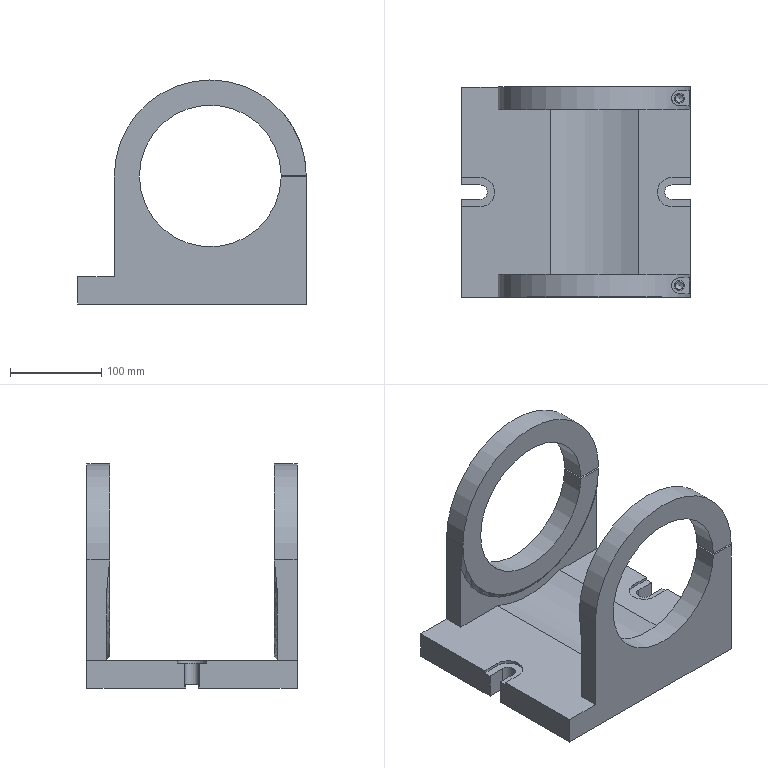Part | NX | features EXTRUDE 14, DATUM_CSYS 12, SKETCH 11, BLEND 4, EXTRACT_STRING 4, REPLACE_FACE 3, UNITE 3, HOLE PACKAGE 2, SIMPLE HOLE 2, SYMBOLIC_THREAD 2, Container 1, DATUM_PLANE 1, EXTRACT_BODY 1, Geometry Instance 1, Instance Feature 1, Mirror Feature 1, SPLIT BODY 1, SUBTRACT 1, TRIM BODY 1 | 1 solid | 78 faces | box 250 x 230 x 245 mm | volume 2370933 mm3 | plane 47 | cylinder 23 | torus 6 | cone 2 | commonest cylinder face diameters 16 x6 10 x4 8.5 x2 11 x2 17 x2 32 x2